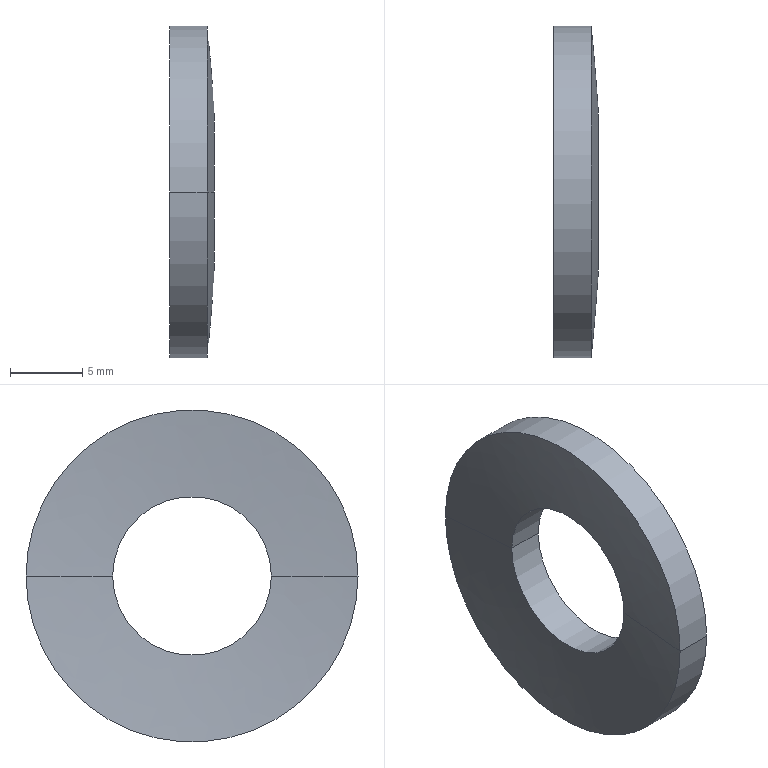Part | STEP file | M10_PAINE_LAATTA | 1 solid | 8 faces | box 3.1 x 23 x 23 mm | volume 834.027 mm3 | spline 4 | cylinder 4 | commonest cylinder face diameters 11 x2 23 x2
STEP:
#1=CARTESIAN_POINT('',(0.,0.,0.));
#2=DIRECTION('',(0.,0.,1.));
#3=DIRECTION('',(1.,0.,0.));
#4=AXIS2_PLACEMENT_3D('',#1,#2,#3);
#5=CARTESIAN_POINT('',(0.,11.5,0.));
#6=VERTEX_POINT('',#5);
#7=CARTESIAN_POINT('',(0.5,5.5,0.));
#8=VERTEX_POINT('',#7);
#9=CARTESIAN_POINT('',(-179.103,-6.446,0.));
#10=DIRECTION('',(0.,0.,-1.));
#11=DIRECTION('',(0.995,0.0997,0.));
#12=AXIS2_PLACEMENT_3D('',#9,#10,#11);
#13=CIRCLE('',#12,180.);
#14=CARTESIAN_POINT('',(-0.01205,11.597,-0.7296));
#15=CARTESIAN_POINT('',(0.1975,9.524,-0.5992));
#16=CARTESIAN_POINT('',(0.3708,7.448,-0.4686));
#17=CARTESIAN_POINT('',(0.508,5.369,-0.3378));
#18=CARTESIAN_POINT('',(-0.01205,12.046,6.407));
#19=CARTESIAN_POINT('',(0.1975,9.893,5.262));
#20=CARTESIAN_POINT('',(0.3708,7.736,4.115));
#21=CARTESIAN_POINT('',(0.508,5.577,2.966));
#22=CARTESIAN_POINT('',(-0.01205,7.151,11.62));
#23=CARTESIAN_POINT('',(0.1975,5.873,9.543));
#24=CARTESIAN_POINT('',(0.3708,4.593,7.463));
#25=CARTESIAN_POINT('',(0.508,3.311,5.38));
#26=CARTESIAN_POINT('',(-0.01205,0.,11.62));
#27=CARTESIAN_POINT('',(0.1975,0.,9.543));
#28=CARTESIAN_POINT('',(0.3708,0.,7.463));
#29=CARTESIAN_POINT('',(0.508,0.,5.38));
#30=CARTESIAN_POINT('',(-0.01205,-7.151,11.62));
#31=CARTESIAN_POINT('',(0.1975,-5.873,9.543));
#32=CARTESIAN_POINT('',(0.3708,-4.593,7.463));
#33=CARTESIAN_POINT('',(0.508,-3.311,5.38));
#34=CARTESIAN_POINT('',(-0.01205,-12.046,6.407));
#35=CARTESIAN_POINT('',(0.1975,-9.893,5.262));
#36=CARTESIAN_POINT('',(0.3708,-7.736,4.115));
#37=CARTESIAN_POINT('',(0.508,-5.577,2.966));
#38=CARTESIAN_POINT('',(-0.01205,-11.597,-0.7296));
#39=CARTESIAN_POINT('',(0.1975,-9.524,-0.5992));
#40=CARTESIAN_POINT('',(0.3708,-7.448,-0.4686));
#41=CARTESIAN_POINT('',(0.508,-5.369,-0.3378));
#42=(BOUNDED_SURFACE()B_SPLINE_SURFACE(3,3,((#14,#15,#16,#17),(#18,#19,#20,#21),(#22,#23,#24,#25),(#26,#27,#28,#29),(#30,#31,#32,#33),(#34,#35,#36,#37),(#38,#39,#40,#41)),.UNSPECIFIED.,.F.,.F.,.F.)B_SPLINE_SURFACE_WITH_KNOTS((4,3,4),(4,4),(0.,1.,2.),(0.,1.),.PIECEWISE_BEZIER_KNOTS.)GEOMETRIC_REPRESENTATION_ITEM()RATIONAL_B_SPLINE_SURFACE(((1.187,1.187,1.187,1.187),(0.9377,0.9376,0.9376,0.9377),(0.9377,0.9376,0.9376,0.9377),(1.187,1.187,1.187,1.187),(0.9377,0.9376,0.9376,0.9377),(0.9377,0.9376,0.9376,0.9377),(1.187,1.187,1.187,1.187)))REPRESENTATION_ITEM('')SURFACE());
#43=CARTESIAN_POINT('',(0.04253,0.01923));
#44=CARTESIAN_POINT('',(0.04253,0.9808));
#45=B_SPLINE_CURVE_WITH_KNOTS('',1,(#43,#44),.UNSPECIFIED.,.F.,.F.,(2,2),(0.,0.03345),.PIECEWISE_BEZIER_KNOTS.);
#46=(GEOMETRIC_REPRESENTATION_CONTEXT(2)PARAMETRIC_REPRESENTATION_CONTEXT()REPRESENTATION_CONTEXT('',''));
#47=DEFINITIONAL_REPRESENTATION('',(#45),#46);
#48=PCURVE('',#42,#47);
#49=CARTESIAN_POINT('',(-0.01205,-11.597,0.7296));
#50=CARTESIAN_POINT('',(0.1975,-9.524,0.5992));
#51=CARTESIAN_POINT('',(0.3708,-7.448,0.4686));
#52=CARTESIAN_POINT('',(0.508,-5.369,0.3378));
#53=CARTESIAN_POINT('',(-0.01205,-12.046,-6.407));
#54=CARTESIAN_POINT('',(0.1975,-9.893,-5.262));
#55=CARTESIAN_POINT('',(0.3708,-7.736,-4.115));
#56=CARTESIAN_POINT('',(0.508,-5.577,-2.966));
#57=CARTESIAN_POINT('',(-0.01205,-7.151,-11.62));
#58=CARTESIAN_POINT('',(0.1975,-5.873,-9.543));
#59=CARTESIAN_POINT('',(0.3708,-4.593,-7.463));
#60=CARTESIAN_POINT('',(0.508,-3.311,-5.38));
#61=CARTESIAN_POINT('',(-0.01205,0.,-11.62));
#62=CARTESIAN_POINT('',(0.1975,0.,-9.543));
#63=CARTESIAN_POINT('',(0.3708,0.,-7.463));
#64=CARTESIAN_POINT('',(0.508,0.,-5.38));
#65=CARTESIAN_POINT('',(-0.01205,7.151,-11.62));
#66=CARTESIAN_POINT('',(0.1975,5.873,-9.543));
#67=CARTESIAN_POINT('',(0.3708,4.593,-7.463));
#68=CARTESIAN_POINT('',(0.508,3.311,-5.38));
#69=CARTESIAN_POINT('',(-0.01205,12.046,-6.407));
#70=CARTESIAN_POINT('',(0.1975,9.893,-5.262));
#71=CARTESIAN_POINT('',(0.3708,7.736,-4.115));
#72=CARTESIAN_POINT('',(0.508,5.577,-2.966));
#73=CARTESIAN_POINT('',(-0.01205,11.597,0.7296));
#74=CARTESIAN_POINT('',(0.1975,9.524,0.5992));
#75=CARTESIAN_POINT('',(0.3708,7.448,0.4686));
#76=CARTESIAN_POINT('',(0.508,5.369,0.3378));
#77=(BOUNDED_SURFACE()B_SPLINE_SURFACE(3,3,((#49,#50,#51,#52),(#53,#54,#55,#56),(#57,#58,#59,#60),(#61,#62,#63,#64),(#65,#66,#67,#68),(#69,#70,#71,#72),(#73,#74,#75,#76)),.UNSPECIFIED.,.F.,.F.,.F.)B_SPLINE_SURFACE_WITH_KNOTS((4,3,4),(4,4),(0.,1.,2.),(0.,1.),.PIECEWISE_BEZIER_KNOTS.)GEOMETRIC_REPRESENTATION_ITEM()RATIONAL_B_SPLINE_SURFACE(((1.187,1.187,1.187,1.187),(0.9377,0.9376,0.9376,0.9377),(0.9377,0.9376,0.9376,0.9377),(1.187,1.187,1.187,1.187),(0.9377,0.9376,0.9376,0.9377),(0.9377,0.9376,0.9376,0.9377),(1.187,1.187,1.187,1.187)))REPRESENTATION_ITEM('')SURFACE());
#78=CARTESIAN_POINT('',(1.957,0.01923));
#79=CARTESIAN_POINT('',(1.957,0.9808));
#80=B_SPLINE_CURVE_WITH_KNOTS('',1,(#78,#79),.UNSPECIFIED.,.F.,.F.,(2,2),(0.,0.03345),.PIECEWISE_BEZIER_KNOTS.);
#81=(GEOMETRIC_REPRESENTATION_CONTEXT(2)PARAMETRIC_REPRESENTATION_CONTEXT()REPRESENTATION_CONTEXT('',''));
#82=DEFINITIONAL_REPRESENTATION('',(#80),#81);
#83=PCURVE('',#77,#82);
#84=SURFACE_CURVE('',#13,(#48,#83),.PCURVE_S1.);
#85=EDGE_CURVE('',#6,#8,#84,.T.);
#86=ORIENTED_EDGE('',*,*,#85,.F.);
#87=CARTESIAN_POINT('',(0.,-11.5,0.));
#88=VERTEX_POINT('',#87);
#89=CARTESIAN_POINT('',(0.,0.,0.));
#90=DIRECTION('',(1.,0.,0.));
#91=DIRECTION('',(0.,1.,0.));
#92=AXIS2_PLACEMENT_3D('',#89,#90,#91);
#93=CIRCLE('',#92,11.5);
#94=CARTESIAN_POINT('',(0.04253,0.01923));
#95=CARTESIAN_POINT('',(0.07433,0.01923));
#96=CARTESIAN_POINT('',(0.1362,0.01923));
#97=CARTESIAN_POINT('',(0.2248,0.01923));
#98=CARTESIAN_POINT('',(0.3106,0.01923));
#99=CARTESIAN_POINT('',(0.3943,0.01923));
#100=CARTESIAN_POINT('',(0.4769,0.01923));
#101=CARTESIAN_POINT('',(0.5593,0.01923));
#102=CARTESIAN_POINT('',(0.6424,0.01923));
#103=CARTESIAN_POINT('',(0.7268,0.01923));
#104=CARTESIAN_POINT('',(0.8138,0.01923));
#105=CARTESIAN_POINT('',(0.9038,0.01923));
#106=CARTESIAN_POINT('',(1.,0.01923));
#107=CARTESIAN_POINT('',(1.096,0.01923));
#108=CARTESIAN_POINT('',(1.186,0.01923));
#109=CARTESIAN_POINT('',(1.273,0.01923));
#110=CARTESIAN_POINT('',(1.358,0.01923));
#111=CARTESIAN_POINT('',(1.441,0.01923));
#112=CARTESIAN_POINT('',(1.523,0.01923));
#113=CARTESIAN_POINT('',(1.606,0.01923));
#114=CARTESIAN_POINT('',(1.689,0.01923));
#115=CARTESIAN_POINT('',(1.775,0.01923));
#116=CARTESIAN_POINT('',(1.864,0.01923));
#117=CARTESIAN_POINT('',(1.926,0.01923));
#118=CARTESIAN_POINT('',(1.957,0.01923));
#119=B_SPLINE_CURVE_WITH_KNOTS('',3,(#94,#95,#96,#97,#98,#99,#100,#101,#102,#103,#104,#105,#106,#107,#108,#109,#110,#111,#112,#113,#114,#115,#116,#117,#118),.UNSPECIFIED.,.F.,.F.,(4,1,1,1,1,1,1,1,1,1,1,1,1,1,1,1,1,1,1,1,1,1,4),(0.,0.1428,0.2856,0.4284,0.5712,0.714,0.8568,0.9996,1.142,1.285,1.428,1.571,1.714,1.856,1.999,2.142,2.285,2.428,2.57,2.713,2.856,2.999,3.142),.QUASI_UNIFORM_KNOTS.);
#120=(GEOMETRIC_REPRESENTATION_CONTEXT(2)PARAMETRIC_REPRESENTATION_CONTEXT()REPRESENTATION_CONTEXT('',''));
#121=DEFINITIONAL_REPRESENTATION('',(#119),#120);
#122=PCURVE('',#42,#121);
#123=CARTESIAN_POINT('',(-0.155,0.,0.));
#124=DIRECTION('',(1.,0.,0.));
#125=DIRECTION('',(0.,-1.,0.));
#126=AXIS2_PLACEMENT_3D('',#123,#124,#125);
#127=CYLINDRICAL_SURFACE('',#126,11.5);
#128=CARTESIAN_POINT('',(3.142,0.155));
#129=DIRECTION('',(1.,0.));
#130=VECTOR('',#129,1.);
#131=LINE('',#128,#130);
#132=(GEOMETRIC_REPRESENTATION_CONTEXT(2)PARAMETRIC_REPRESENTATION_CONTEXT()REPRESENTATION_CONTEXT('',''));
#133=DEFINITIONAL_REPRESENTATION('',(#131),#132);
#134=PCURVE('',#127,#133);
#135=SURFACE_CURVE('',#93,(#122,#134),.PCURVE_S1.);
#136=EDGE_CURVE('',#6,#88,#135,.T.);
#137=ORIENTED_EDGE('',*,*,#136,.T.);
#138=CARTESIAN_POINT('',(0.5,-5.5,0.));
#139=VERTEX_POINT('',#138);
#140=CARTESIAN_POINT('',(-179.103,6.446,0.));
#141=DIRECTION('',(0.,0.,1.));
#142=DIRECTION('',(0.995,-0.0997,0.));
#143=AXIS2_PLACEMENT_3D('',#140,#141,#142);
#144=CIRCLE('',#143,180.);
#145=CARTESIAN_POINT('',(1.957,0.01923));
#146=CARTESIAN_POINT('',(1.957,0.9808));
#147=B_SPLINE_CURVE_WITH_KNOTS('',1,(#145,#146),.UNSPECIFIED.,.F.,.F.,(2,2),(0.,0.03345),.PIECEWISE_BEZIER_KNOTS.);
#148=(GEOMETRIC_REPRESENTATION_CONTEXT(2)PARAMETRIC_REPRESENTATION_CONTEXT()REPRESENTATION_CONTEXT('',''));
#149=DEFINITIONAL_REPRESENTATION('',(#147),#148);
#150=PCURVE('',#42,#149);
#151=CARTESIAN_POINT('',(0.04253,0.01923));
#152=CARTESIAN_POINT('',(0.04253,0.9808));
#153=B_SPLINE_CURVE_WITH_KNOTS('',1,(#151,#152),.UNSPECIFIED.,.F.,.F.,(2,2),(0.,0.03345),.PIECEWISE_BEZIER_KNOTS.);
#154=(GEOMETRIC_REPRESENTATION_CONTEXT(2)PARAMETRIC_REPRESENTATION_CONTEXT()REPRESENTATION_CONTEXT('',''));
#155=DEFINITIONAL_REPRESENTATION('',(#153),#154);
#156=PCURVE('',#77,#155);
#157=SURFACE_CURVE('',#144,(#150,#156),.PCURVE_S1.);
#158=EDGE_CURVE('',#88,#139,#157,.T.);
#159=ORIENTED_EDGE('',*,*,#158,.T.);
#160=CARTESIAN_POINT('',(0.5,0.,0.));
#161=DIRECTION('',(1.,0.,0.));
#162=DIRECTION('',(0.,1.,0.));
#163=AXIS2_PLACEMENT_3D('',#160,#161,#162);
#164=CIRCLE('',#163,5.5);
#165=CARTESIAN_POINT('',(0.04253,0.9808));
#166=CARTESIAN_POINT('',(0.07433,0.9808));
#167=CARTESIAN_POINT('',(0.1362,0.9808));
#168=CARTESIAN_POINT('',(0.2248,0.9808));
#169=CARTESIAN_POINT('',(0.3106,0.9808));
#170=CARTESIAN_POINT('',(0.3943,0.9808));
#171=CARTESIAN_POINT('',(0.4769,0.9808));
#172=CARTESIAN_POINT('',(0.5593,0.9808));
#173=CARTESIAN_POINT('',(0.6424,0.9808));
#174=CARTESIAN_POINT('',(0.7268,0.9808));
#175=CARTESIAN_POINT('',(0.8138,0.9808));
#176=CARTESIAN_POINT('',(0.9038,0.9808));
#177=CARTESIAN_POINT('',(1.,0.9808));
#178=CARTESIAN_POINT('',(1.096,0.9808));
#179=CARTESIAN_POINT('',(1.186,0.9808));
#180=CARTESIAN_POINT('',(1.273,0.9808));
#181=CARTESIAN_POINT('',(1.358,0.9808));
#182=CARTESIAN_POINT('',(1.441,0.9808));
#183=CARTESIAN_POINT('',(1.523,0.9808));
#184=CARTESIAN_POINT('',(1.606,0.9808));
#185=CARTESIAN_POINT('',(1.689,0.9808));
#186=CARTESIAN_POINT('',(1.775,0.9808));
#187=CARTESIAN_POINT('',(1.864,0.9808));
#188=CARTESIAN_POINT('',(1.926,0.9808));
#189=CARTESIAN_POINT('',(1.957,0.9808));
#190=B_SPLINE_CURVE_WITH_KNOTS('',3,(#165,#166,#167,#168,#169,#170,#171,#172,#173,#174,#175,#176,#177,#178,#179,#180,#181,#182,#183,#184,#185,#186,#187,#188,#189),.UNSPECIFIED.,.F.,.F.,(4,1,1,1,1,1,1,1,1,1,1,1,1,1,1,1,1,1,1,1,1,1,4),(0.,0.1428,0.2856,0.4284,0.5712,0.714,0.8568,0.9996,1.142,1.285,1.428,1.571,1.714,1.856,1.999,2.142,2.285,2.428,2.57,2.713,2.856,2.999,3.142),.QUASI_UNIFORM_KNOTS.);
#191=(GEOMETRIC_REPRESENTATION_CONTEXT(2)PARAMETRIC_REPRESENTATION_CONTEXT()REPRESENTATION_CONTEXT('',''));
#192=DEFINITIONAL_REPRESENTATION('',(#190),#191);
#193=PCURVE('',#42,#192);
#194=CARTESIAN_POINT('',(-0.155,0.,0.));
#195=DIRECTION('',(1.,0.,0.));
#196=DIRECTION('',(0.,-1.,0.));
#197=AXIS2_PLACEMENT_3D('',#194,#195,#196);
#198=CYLINDRICAL_SURFACE('',#197,5.5);
#199=CARTESIAN_POINT('',(3.142,0.655));
#200=DIRECTION('',(1.,0.));
#201=VECTOR('',#200,1.);
#202=LINE('',#199,#201);
#203=(GEOMETRIC_REPRESENTATION_CONTEXT(2)PARAMETRIC_REPRESENTATION_CONTEXT()REPRESENTATION_CONTEXT('',''));
#204=DEFINITIONAL_REPRESENTATION('',(#202),#203);
#205=PCURVE('',#198,#204);
#206=SURFACE_CURVE('',#164,(#193,#205),.PCURVE_S1.);
#207=EDGE_CURVE('',#8,#139,#206,.T.);
#208=ORIENTED_EDGE('',*,*,#207,.F.);
#209=EDGE_LOOP('',(#86,#137,#159,#208));
#210=FACE_BOUND('',#209,.F.);
#211=ADVANCED_FACE('',(#210),#42,.F.);
#212=ORIENTED_EDGE('',*,*,#85,.T.);
#213=CARTESIAN_POINT('',(0.5,0.,0.));
#214=DIRECTION('',(-1.,0.,0.));
#215=DIRECTION('',(0.,1.,0.));
#216=AXIS2_PLACEMENT_3D('',#213,#214,#215);
#217=CIRCLE('',#216,5.5);
#218=CARTESIAN_POINT('',(1.957,0.9808));
#219=CARTESIAN_POINT('',(1.926,0.9808));
#220=CARTESIAN_POINT('',(1.864,0.9808));
#221=CARTESIAN_POINT('',(1.775,0.9808));
#222=CARTESIAN_POINT('',(1.689,0.9808));
#223=CARTESIAN_POINT('',(1.606,0.9808));
#224=CARTESIAN_POINT('',(1.523,0.9808));
#225=CARTESIAN_POINT('',(1.441,0.9808));
#226=CARTESIAN_POINT('',(1.358,0.9808));
#227=CARTESIAN_POINT('',(1.273,0.9808));
#228=CARTESIAN_POINT('',(1.186,0.9808));
#229=CARTESIAN_POINT('',(1.096,0.9808));
#230=CARTESIAN_POINT('',(1.,0.9808));
#231=CARTESIAN_POINT('',(0.9038,0.9808));
#232=CARTESIAN_POINT('',(0.8138,0.9808));
#233=CARTESIAN_POINT('',(0.7268,0.9808));
#234=CARTESIAN_POINT('',(0.6424,0.9808));
#235=CARTESIAN_POINT('',(0.5593,0.9808));
#236=CARTESIAN_POINT('',(0.4769,0.9808));
#237=CARTESIAN_POINT('',(0.3943,0.9808));
#238=CARTESIAN_POINT('',(0.3106,0.9808));
#239=CARTESIAN_POINT('',(0.2248,0.9808));
#240=CARTESIAN_POINT('',(0.1362,0.9808));
#241=CARTESIAN_POINT('',(0.07433,0.9808));
#242=CARTESIAN_POINT('',(0.04253,0.9808));
#243=B_SPLINE_CURVE_WITH_KNOTS('',3,(#218,#219,#220,#221,#222,#223,#224,#225,#226,#227,#228,#229,#230,#231,#232,#233,#234,#235,#236,#237,#238,#239,#240,#241,#242),.UNSPECIFIED.,.F.,.F.,(4,1,1,1,1,1,1,1,1,1,1,1,1,1,1,1,1,1,1,1,1,1,4),(0.,0.1428,0.2856,0.4284,0.5712,0.714,0.8568,0.9996,1.142,1.285,1.428,1.571,1.714,1.856,1.999,2.142,2.285,2.428,2.57,2.713,2.856,2.999,3.142),.QUASI_UNIFORM_KNOTS.);
#244=(GEOMETRIC_REPRESENTATION_CONTEXT(2)PARAMETRIC_REPRESENTATION_CONTEXT()REPRESENTATION_CONTEXT('',''));
#245=DEFINITIONAL_REPRESENTATION('',(#243),#244);
#246=PCURVE('',#77,#245);
#247=CARTESIAN_POINT('',(-0.155,0.,0.));
#248=DIRECTION('',(1.,0.,0.));
#249=DIRECTION('',(0.,-1.,0.));
#250=AXIS2_PLACEMENT_3D('',#247,#248,#249);
#251=CYLINDRICAL_SURFACE('',#250,5.5);
#252=CARTESIAN_POINT('',(3.142,0.655));
#253=DIRECTION('',(-1.,0.));
#254=VECTOR('',#253,1.);
#255=LINE('',#252,#254);
#256=(GEOMETRIC_REPRESENTATION_CONTEXT(2)PARAMETRIC_REPRESENTATION_CONTEXT()REPRESENTATION_CONTEXT('',''));
#257=DEFINITIONAL_REPRESENTATION('',(#255),#256);
#258=PCURVE('',#251,#257);
#259=SURFACE_CURVE('',#217,(#246,#258),.PCURVE_S1.);
#260=EDGE_CURVE('',#8,#139,#259,.T.);
#261=ORIENTED_EDGE('',*,*,#260,.T.);
#262=ORIENTED_EDGE('',*,*,#158,.F.);
#263=CARTESIAN_POINT('',(0.,0.,0.));
#264=DIRECTION('',(-1.,0.,0.));
#265=DIRECTION('',(0.,1.,0.));
#266=AXIS2_PLACEMENT_3D('',#263,#264,#265);
#267=CIRCLE('',#266,11.5);
#268=CARTESIAN_POINT('',(1.957,0.01923));
#269=CARTESIAN_POINT('',(1.926,0.01923));
#270=CARTESIAN_POINT('',(1.864,0.01923));
#271=CARTESIAN_POINT('',(1.775,0.01923));
#272=CARTESIAN_POINT('',(1.689,0.01923));
#273=CARTESIAN_POINT('',(1.606,0.01923));
#274=CARTESIAN_POINT('',(1.523,0.01923));
#275=CARTESIAN_POINT('',(1.441,0.01923));
#276=CARTESIAN_POINT('',(1.358,0.01923));
#277=CARTESIAN_POINT('',(1.273,0.01923));
#278=CARTESIAN_POINT('',(1.186,0.01923));
#279=CARTESIAN_POINT('',(1.096,0.01923));
#280=CARTESIAN_POINT('',(1.,0.01923));
#281=CARTESIAN_POINT('',(0.9038,0.01923));
#282=CARTESIAN_POINT('',(0.8138,0.01923));
#283=CARTESIAN_POINT('',(0.7268,0.01923));
#284=CARTESIAN_POINT('',(0.6424,0.01923));
#285=CARTESIAN_POINT('',(0.5593,0.01923));
#286=CARTESIAN_POINT('',(0.4769,0.01923));
#287=CARTESIAN_POINT('',(0.3943,0.01923));
#288=CARTESIAN_POINT('',(0.3106,0.01923));
#289=CARTESIAN_POINT('',(0.2248,0.01923));
#290=CARTESIAN_POINT('',(0.1362,0.01923));
#291=CARTESIAN_POINT('',(0.07433,0.01923));
#292=CARTESIAN_POINT('',(0.04253,0.01923));
#293=B_SPLINE_CURVE_WITH_KNOTS('',3,(#268,#269,#270,#271,#272,#273,#274,#275,#276,#277,#278,#279,#280,#281,#282,#283,#284,#285,#286,#287,#288,#289,#290,#291,#292),.UNSPECIFIED.,.F.,.F.,(4,1,1,1,1,1,1,1,1,1,1,1,1,1,1,1,1,1,1,1,1,1,4),(0.,0.1428,0.2856,0.4284,0.5712,0.714,0.8568,0.9996,1.142,1.285,1.428,1.571,1.714,1.856,1.999,2.142,2.285,2.428,2.57,2.713,2.856,2.999,3.142),.QUASI_UNIFORM_KNOTS.);
#294=(GEOMETRIC_REPRESENTATION_CONTEXT(2)PARAMETRIC_REPRESENTATION_CONTEXT()REPRESENTATION_CONTEXT('',''));
#295=DEFINITIONAL_REPRESENTATION('',(#293),#294);
#296=PCURVE('',#77,#295);
#297=CARTESIAN_POINT('',(-0.155,0.,0.));
#298=DIRECTION('',(1.,0.,0.));
#299=DIRECTION('',(0.,-1.,0.));
#300=AXIS2_PLACEMENT_3D('',#297,#298,#299);
#301=CYLINDRICAL_SURFACE('',#300,11.5);
#302=CARTESIAN_POINT('',(3.142,0.155));
#303=DIRECTION('',(-1.,0.));
#304=VECTOR('',#303,1.);
#305=LINE('',#302,#304);
#306=(GEOMETRIC_REPRESENTATION_CONTEXT(2)PARAMETRIC_REPRESENTATION_CONTEXT()REPRESENTATION_CONTEXT('',''));
#307=DEFINITIONAL_REPRESENTATION('',(#305),#306);
#308=PCURVE('',#301,#307);
#309=SURFACE_CURVE('',#267,(#296,#308),.PCURVE_S1.);
#310=EDGE_CURVE('',#6,#88,#309,.T.);
#311=ORIENTED_EDGE('',*,*,#310,.F.);
#312=EDGE_LOOP('',(#212,#261,#262,#311));
#313=FACE_BOUND('',#312,.F.);
#314=ADVANCED_FACE('',(#313),#77,.F.);
#315=CARTESIAN_POINT('',(3.1,5.5,0.));
#316=VERTEX_POINT('',#315);
#317=CARTESIAN_POINT('',(0.5,5.5,0.));
#318=DIRECTION('',(1.,0.,0.));
#319=VECTOR('',#318,1.);
#320=LINE('',#317,#319);
#321=CARTESIAN_POINT('',(3.142,0.655));
#322=DIRECTION('',(0.,1.));
#323=VECTOR('',#322,1.);
#324=LINE('',#321,#323);
#325=(GEOMETRIC_REPRESENTATION_CONTEXT(2)PARAMETRIC_REPRESENTATION_CONTEXT()REPRESENTATION_CONTEXT('',''));
#326=DEFINITIONAL_REPRESENTATION('',(#324),#325);
#327=PCURVE('',#251,#326);
#328=CARTESIAN_POINT('',(3.142,0.655));
#329=DIRECTION('',(0.,1.));
#330=VECTOR('',#329,1.);
#331=LINE('',#328,#330);
#332=(GEOMETRIC_REPRESENTATION_CONTEXT(2)PARAMETRIC_REPRESENTATION_CONTEXT()REPRESENTATION_CONTEXT('',''));
#333=DEFINITIONAL_REPRESENTATION('',(#331),#332);
#334=PCURVE('',#198,#333);
#335=SURFACE_CURVE('',#320,(#327,#334),.PCURVE_S1.);
#336=EDGE_CURVE('',#8,#316,#335,.T.);
#337=ORIENTED_EDGE('',*,*,#336,.T.);
#338=CARTESIAN_POINT('',(3.1,-5.5,0.));
#339=VERTEX_POINT('',#338);
#340=CARTESIAN_POINT('',(3.1,0.,0.));
#341=DIRECTION('',(-1.,0.,0.));
#342=DIRECTION('',(0.,1.,0.));
#343=AXIS2_PLACEMENT_3D('',#340,#341,#342);
#344=CIRCLE('',#343,5.5);
#345=CARTESIAN_POINT('',(3.142,3.255));
#346=DIRECTION('',(-1.,0.));
#347=VECTOR('',#346,1.);
#348=LINE('',#345,#347);
#349=(GEOMETRIC_REPRESENTATION_CONTEXT(2)PARAMETRIC_REPRESENTATION_CONTEXT()REPRESENTATION_CONTEXT('',''));
#350=DEFINITIONAL_REPRESENTATION('',(#348),#349);
#351=PCURVE('',#251,#350);
#352=CARTESIAN_POINT('',(2.588,-11.597,0.7296));
#353=CARTESIAN_POINT('',(2.797,-9.524,0.5992));
#354=CARTESIAN_POINT('',(2.971,-7.448,0.4686));
#355=CARTESIAN_POINT('',(3.108,-5.369,0.3378));
#356=CARTESIAN_POINT('',(2.588,-12.046,-6.407));
#357=CARTESIAN_POINT('',(2.797,-9.893,-5.262));
#358=CARTESIAN_POINT('',(2.971,-7.736,-4.115));
#359=CARTESIAN_POINT('',(3.108,-5.577,-2.966));
#360=CARTESIAN_POINT('',(2.588,-7.151,-11.62));
#361=CARTESIAN_POINT('',(2.797,-5.873,-9.543));
#362=CARTESIAN_POINT('',(2.971,-4.593,-7.463));
#363=CARTESIAN_POINT('',(3.108,-3.311,-5.38));
#364=CARTESIAN_POINT('',(2.588,0.,-11.62));
#365=CARTESIAN_POINT('',(2.797,0.,-9.543));
#366=CARTESIAN_POINT('',(2.971,0.,-7.463));
#367=CARTESIAN_POINT('',(3.108,0.,-5.38));
#368=CARTESIAN_POINT('',(2.588,7.151,-11.62));
#369=CARTESIAN_POINT('',(2.797,5.873,-9.543));
#370=CARTESIAN_POINT('',(2.971,4.593,-7.463));
#371=CARTESIAN_POINT('',(3.108,3.311,-5.38));
#372=CARTESIAN_POINT('',(2.588,12.046,-6.407));
#373=CARTESIAN_POINT('',(2.797,9.893,-5.262));
#374=CARTESIAN_POINT('',(2.971,7.736,-4.115));
#375=CARTESIAN_POINT('',(3.108,5.577,-2.966));
#376=CARTESIAN_POINT('',(2.588,11.597,0.7296));
#377=CARTESIAN_POINT('',(2.797,9.524,0.5992));
#378=CARTESIAN_POINT('',(2.971,7.448,0.4686));
#379=CARTESIAN_POINT('',(3.108,5.369,0.3378));
#380=(BOUNDED_SURFACE()B_SPLINE_SURFACE(3,3,((#352,#353,#354,#355),(#356,#357,#358,#359),(#360,#361,#362,#363),(#364,#365,#366,#367),(#368,#369,#370,#371),(#372,#373,#374,#375),(#376,#377,#378,#379)),.UNSPECIFIED.,.F.,.F.,.F.)B_SPLINE_SURFACE_WITH_KNOTS((4,3,4),(4,4),(0.,1.,2.),(0.,1.),.PIECEWISE_BEZIER_KNOTS.)GEOMETRIC_REPRESENTATION_ITEM()RATIONAL_B_SPLINE_SURFACE(((1.187,1.187,1.187,1.187),(0.9377,0.9376,0.9376,0.9377),(0.9377,0.9376,0.9376,0.9377),(1.187,1.187,1.187,1.187),(0.9377,0.9376,0.9376,0.9377),(0.9377,0.9376,0.9376,0.9377),(1.187,1.187,1.187,1.187)))REPRESENTATION_ITEM('')SURFACE());
#381=CARTESIAN_POINT('',(1.957,0.9808));
#382=CARTESIAN_POINT('',(1.926,0.9808));
#383=CARTESIAN_POINT('',(1.864,0.9808));
#384=CARTESIAN_POINT('',(1.775,0.9808));
#385=CARTESIAN_POINT('',(1.689,0.9808));
#386=CARTESIAN_POINT('',(1.606,0.9808));
#387=CARTESIAN_POINT('',(1.523,0.9808));
#388=CARTESIAN_POINT('',(1.441,0.9808));
#389=CARTESIAN_POINT('',(1.358,0.9808));
#390=CARTESIAN_POINT('',(1.273,0.9808));
#391=CARTESIAN_POINT('',(1.186,0.9808));
#392=CARTESIAN_POINT('',(1.096,0.9808));
#393=CARTESIAN_POINT('',(1.,0.9808));
#394=CARTESIAN_POINT('',(0.9038,0.9808));
#395=CARTESIAN_POINT('',(0.8138,0.9808));
#396=CARTESIAN_POINT('',(0.7268,0.9808));
#397=CARTESIAN_POINT('',(0.6424,0.9808));
#398=CARTESIAN_POINT('',(0.5593,0.9808));
#399=CARTESIAN_POINT('',(0.4769,0.9808));
#400=CARTESIAN_POINT('',(0.3943,0.9808));
#401=CARTESIAN_POINT('',(0.3106,0.9808));
#402=CARTESIAN_POINT('',(0.2248,0.9808));
#403=CARTESIAN_POINT('',(0.1362,0.9808));
#404=CARTESIAN_POINT('',(0.07433,0.9808));
#405=CARTESIAN_POINT('',(0.04253,0.9808));
#406=B_SPLINE_CURVE_WITH_KNOTS('',3,(#381,#382,#383,#384,#385,#386,#387,#388,#389,#390,#391,#392,#393,#394,#395,#396,#397,#398,#399,#400,#401,#402,#403,#404,#405),.UNSPECIFIED.,.F.,.F.,(4,1,1,1,1,1,1,1,1,1,1,1,1,1,1,1,1,1,1,1,1,1,4),(0.,0.1428,0.2856,0.4284,0.5712,0.714,0.8568,0.9996,1.142,1.285,1.428,1.571,1.714,1.856,1.999,2.142,2.285,2.428,2.57,2.713,2.856,2.999,3.142),.QUASI_UNIFORM_KNOTS.);
#407=(GEOMETRIC_REPRESENTATION_CONTEXT(2)PARAMETRIC_REPRESENTATION_CONTEXT()REPRESENTATION_CONTEXT('',''));
#408=DEFINITIONAL_REPRESENTATION('',(#406),#407);
#409=PCURVE('',#380,#408);
#410=SURFACE_CURVE('',#344,(#351,#409),.PCURVE_S1.);
#411=EDGE_CURVE('',#316,#339,#410,.T.);
#412=ORIENTED_EDGE('',*,*,#411,.T.);
#413=CARTESIAN_POINT('',(0.5,-5.5,0.));
#414=DIRECTION('',(1.,0.,0.));
#415=VECTOR('',#414,1.);
#416=LINE('',#413,#415);
#417=CARTESIAN_POINT('',(0.,0.655));
#418=DIRECTION('',(0.,1.));
#419=VECTOR('',#418,1.);
#420=LINE('',#417,#419);
#421=(GEOMETRIC_REPRESENTATION_CONTEXT(2)PARAMETRIC_REPRESENTATION_CONTEXT()REPRESENTATION_CONTEXT('',''));
#422=DEFINITIONAL_REPRESENTATION('',(#420),#421);
#423=PCURVE('',#251,#422);
#424=CARTESIAN_POINT('',(6.283,0.655));
#425=DIRECTION('',(0.,1.));
#426=VECTOR('',#425,1.);
#427=LINE('',#424,#426);
#428=(GEOMETRIC_REPRESENTATION_CONTEXT(2)PARAMETRIC_REPRESENTATION_CONTEXT()REPRESENTATION_CONTEXT('',''));
#429=DEFINITIONAL_REPRESENTATION('',(#427),#428);
#430=PCURVE('',#198,#429);
#431=SURFACE_CURVE('',#416,(#423,#430),.PCURVE_S1.);
#432=EDGE_CURVE('',#139,#339,#431,.T.);
#433=ORIENTED_EDGE('',*,*,#432,.F.);
#434=ORIENTED_EDGE('',*,*,#260,.F.);
#435=EDGE_LOOP('',(#337,#412,#433,#434));
#436=FACE_BOUND('',#435,.F.);
#437=ADVANCED_FACE('',(#436),#251,.F.);
#438=ORIENTED_EDGE('',*,*,#336,.F.);
#439=ORIENTED_EDGE('',*,*,#207,.T.);
#440=ORIENTED_EDGE('',*,*,#432,.T.);
#441=CARTESIAN_POINT('',(3.1,0.,0.));
#442=DIRECTION('',(1.,0.,0.));
#443=DIRECTION('',(0.,1.,0.));
#444=AXIS2_PLACEMENT_3D('',#441,#442,#443);
#445=CIRCLE('',#444,5.5);
#446=CARTESIAN_POINT('',(3.142,3.255));
#447=DIRECTION('',(1.,0.));
#448=VECTOR('',#447,1.);
#449=LINE('',#446,#448);
#450=(GEOMETRIC_REPRESENTATION_CONTEXT(2)PARAMETRIC_REPRESENTATION_CONTEXT()REPRESENTATION_CONTEXT('',''));
#451=DEFINITIONAL_REPRESENTATION('',(#449),#450);
#452=PCURVE('',#198,#451);
#453=CARTESIAN_POINT('',(2.588,11.597,-0.7296));
#454=CARTESIAN_POINT('',(2.797,9.524,-0.5992));
#455=CARTESIAN_POINT('',(2.971,7.448,-0.4686));
#456=CARTESIAN_POINT('',(3.108,5.369,-0.3378));
#457=CARTESIAN_POINT('',(2.588,12.046,6.407));
#458=CARTESIAN_POINT('',(2.797,9.893,5.262));
#459=CARTESIAN_POINT('',(2.971,7.736,4.115));
#460=CARTESIAN_POINT('',(3.108,5.577,2.966));
#461=CARTESIAN_POINT('',(2.588,7.151,11.62));
#462=CARTESIAN_POINT('',(2.797,5.873,9.543));
#463=CARTESIAN_POINT('',(2.971,4.593,7.463));
#464=CARTESIAN_POINT('',(3.108,3.311,5.38));
#465=CARTESIAN_POINT('',(2.588,0.,11.62));
#466=CARTESIAN_POINT('',(2.797,0.,9.543));
#467=CARTESIAN_POINT('',(2.971,0.,7.463));
#468=CARTESIAN_POINT('',(3.108,0.,5.38));
#469=CARTESIAN_POINT('',(2.588,-7.151,11.62));
#470=CARTESIAN_POINT('',(2.797,-5.873,9.543));
#471=CARTESIAN_POINT('',(2.971,-4.593,7.463));
#472=CARTESIAN_POINT('',(3.108,-3.311,5.38));
#473=CARTESIAN_POINT('',(2.588,-12.046,6.407));
#474=CARTESIAN_POINT('',(2.797,-9.893,5.262));
#475=CARTESIAN_POINT('',(2.971,-7.736,4.115));
#476=CARTESIAN_POINT('',(3.108,-5.577,2.966));
#477=CARTESIAN_POINT('',(2.588,-11.597,-0.7296));
#478=CARTESIAN_POINT('',(2.797,-9.524,-0.5992));
#479=CARTESIAN_POINT('',(2.971,-7.448,-0.4686));
#480=CARTESIAN_POINT('',(3.108,-5.369,-0.3378));
#481=(BOUNDED_SURFACE()B_SPLINE_SURFACE(3,3,((#453,#454,#455,#456),(#457,#458,#459,#460),(#461,#462,#463,#464),(#465,#466,#467,#468),(#469,#470,#471,#472),(#473,#474,#475,#476),(#477,#478,#479,#480)),.UNSPECIFIED.,.F.,.F.,.F.)B_SPLINE_SURFACE_WITH_KNOTS((4,3,4),(4,4),(0.,1.,2.),(0.,1.),.PIECEWISE_BEZIER_KNOTS.)GEOMETRIC_REPRESENTATION_ITEM()RATIONAL_B_SPLINE_SURFACE(((1.187,1.187,1.187,1.187),(0.9377,0.9376,0.9376,0.9377),(0.9377,0.9376,0.9376,0.9377),(1.187,1.187,1.187,1.187),(0.9377,0.9376,0.9376,0.9377),(0.9377,0.9376,0.9376,0.9377),(1.187,1.187,1.187,1.187)))REPRESENTATION_ITEM('')SURFACE());
#482=CARTESIAN_POINT('',(0.04253,0.9808));
#483=CARTESIAN_POINT('',(0.07433,0.9808));
#484=CARTESIAN_POINT('',(0.1362,0.9808));
#485=CARTESIAN_POINT('',(0.2248,0.9808));
#486=CARTESIAN_POINT('',(0.3106,0.9808));
#487=CARTESIAN_POINT('',(0.3943,0.9808));
#488=CARTESIAN_POINT('',(0.4769,0.9808));
#489=CARTESIAN_POINT('',(0.5593,0.9808));
#490=CARTESIAN_POINT('',(0.6424,0.9808));
#491=CARTESIAN_POINT('',(0.7268,0.9808));
#492=CARTESIAN_POINT('',(0.8138,0.9808));
#493=CARTESIAN_POINT('',(0.9038,0.9808));
#494=CARTESIAN_POINT('',(1.,0.9808));
#495=CARTESIAN_POINT('',(1.096,0.9808));
#496=CARTESIAN_POINT('',(1.186,0.9808));
#497=CARTESIAN_POINT('',(1.273,0.9808));
#498=CARTESIAN_POINT('',(1.358,0.9808));
#499=CARTESIAN_POINT('',(1.441,0.9808));
#500=CARTESIAN_POINT('',(1.523,0.9808));
#501=CARTESIAN_POINT('',(1.606,0.9808));
#502=CARTESIAN_POINT('',(1.689,0.9808));
#503=CARTESIAN_POINT('',(1.775,0.9808));
#504=CARTESIAN_POINT('',(1.864,0.9808));
#505=CARTESIAN_POINT('',(1.926,0.9808));
#506=CARTESIAN_POINT('',(1.957,0.9808));
#507=B_SPLINE_CURVE_WITH_KNOTS('',3,(#482,#483,#484,#485,#486,#487,#488,#489,#490,#491,#492,#493,#494,#495,#496,#497,#498,#499,#500,#501,#502,#503,#504,#505,#506),.UNSPECIFIED.,.F.,.F.,(4,1,1,1,1,1,1,1,1,1,1,1,1,1,1,1,1,1,1,1,1,1,4),(0.,0.1428,0.2856,0.4284,0.5712,0.714,0.8568,0.9996,1.142,1.285,1.428,1.571,1.714,1.856,1.999,2.142,2.285,2.428,2.57,2.713,2.856,2.999,3.142),.QUASI_UNIFORM_KNOTS.);
#508=(GEOMETRIC_REPRESENTATION_CONTEXT(2)PARAMETRIC_REPRESENTATION_CONTEXT()REPRESENTATION_CONTEXT('',''));
#509=DEFINITIONAL_REPRESENTATION('',(#507),#508);
#510=PCURVE('',#481,#509);
#511=SURFACE_CURVE('',#445,(#452,#510),.PCURVE_S1.);
#512=EDGE_CURVE('',#316,#339,#511,.T.);
#513=ORIENTED_EDGE('',*,*,#512,.F.);
#514=EDGE_LOOP('',(#438,#439,#440,#513));
#515=FACE_BOUND('',#514,.F.);
#516=ADVANCED_FACE('',(#515),#198,.F.);
#517=CARTESIAN_POINT('',(2.6,11.5,0.));
#518=VERTEX_POINT('',#517);
#519=CARTESIAN_POINT('',(2.6,-11.5,0.));
#520=VERTEX_POINT('',#519);
#521=CARTESIAN_POINT('',(2.6,0.,0.));
#522=DIRECTION('',(1.,0.,0.));
#523=DIRECTION('',(0.,1.,0.));
#524=AXIS2_PLACEMENT_3D('',#521,#522,#523);
#525=CIRCLE('',#524,11.5);
#526=CARTESIAN_POINT('',(0.04253,0.01923));
#527=CARTESIAN_POINT('',(0.07433,0.01923));
#528=CARTESIAN_POINT('',(0.1362,0.01923));
#529=CARTESIAN_POINT('',(0.2248,0.01923));
#530=CARTESIAN_POINT('',(0.3106,0.01923));
#531=CARTESIAN_POINT('',(0.3943,0.01923));
#532=CARTESIAN_POINT('',(0.4769,0.01923));
#533=CARTESIAN_POINT('',(0.5593,0.01923));
#534=CARTESIAN_POINT('',(0.6424,0.01923));
#535=CARTESIAN_POINT('',(0.7268,0.01923));
#536=CARTESIAN_POINT('',(0.8138,0.01923));
#537=CARTESIAN_POINT('',(0.9038,0.01923));
#538=CARTESIAN_POINT('',(1.,0.01923));
#539=CARTESIAN_POINT('',(1.096,0.01923));
#540=CARTESIAN_POINT('',(1.186,0.01923));
#541=CARTESIAN_POINT('',(1.273,0.01923));
#542=CARTESIAN_POINT('',(1.358,0.01923));
#543=CARTESIAN_POINT('',(1.441,0.01923));
#544=CARTESIAN_POINT('',(1.523,0.01923));
#545=CARTESIAN_POINT('',(1.606,0.01923));
#546=CARTESIAN_POINT('',(1.689,0.01923));
#547=CARTESIAN_POINT('',(1.775,0.01923));
#548=CARTESIAN_POINT('',(1.864,0.01923));
#549=CARTESIAN_POINT('',(1.926,0.01923));
#550=CARTESIAN_POINT('',(1.957,0.01923));
#551=B_SPLINE_CURVE_WITH_KNOTS('',3,(#526,#527,#528,#529,#530,#531,#532,#533,#534,#535,#536,#537,#538,#539,#540,#541,#542,#543,#544,#545,#546,#547,#548,#549,#550),.UNSPECIFIED.,.F.,.F.,(4,1,1,1,1,1,1,1,1,1,1,1,1,1,1,1,1,1,1,1,1,1,4),(0.,0.1428,0.2856,0.4284,0.5712,0.714,0.8568,0.9996,1.142,1.285,1.428,1.571,1.714,1.856,1.999,2.142,2.285,2.428,2.57,2.713,2.856,2.999,3.142),.QUASI_UNIFORM_KNOTS.);
#552=(GEOMETRIC_REPRESENTATION_CONTEXT(2)PARAMETRIC_REPRESENTATION_CONTEXT()REPRESENTATION_CONTEXT('',''));
#553=DEFINITIONAL_REPRESENTATION('',(#551),#552);
#554=PCURVE('',#481,#553);
#555=CARTESIAN_POINT('',(3.142,2.755));
#556=DIRECTION('',(1.,0.));
#557=VECTOR('',#556,1.);
#558=LINE('',#555,#557);
#559=(GEOMETRIC_REPRESENTATION_CONTEXT(2)PARAMETRIC_REPRESENTATION_CONTEXT()REPRESENTATION_CONTEXT('',''));
#560=DEFINITIONAL_REPRESENTATION('',(#558),#559);
#561=PCURVE('',#127,#560);
#562=SURFACE_CURVE('',#525,(#554,#561),.PCURVE_S1.);
#563=EDGE_CURVE('',#518,#520,#562,.T.);
#564=ORIENTED_EDGE('',*,*,#563,.T.);
#565=CARTESIAN_POINT('',(-176.503,6.446,0.));
#566=DIRECTION('',(0.,0.,-1.));
#567=DIRECTION('',(0.9978,-0.06637,0.));
#568=AXIS2_PLACEMENT_3D('',#565,#566,#567);
#569=CIRCLE('',#568,180.);
#570=CARTESIAN_POINT('',(1.957,0.9808));
#571=CARTESIAN_POINT('',(1.957,0.01923));
#572=B_SPLINE_CURVE_WITH_KNOTS('',1,(#570,#571),.UNSPECIFIED.,.F.,.F.,(2,2),(0.,0.03345),.PIECEWISE_BEZIER_KNOTS.);
#573=(GEOMETRIC_REPRESENTATION_CONTEXT(2)PARAMETRIC_REPRESENTATION_CONTEXT()REPRESENTATION_CONTEXT('',''));
#574=DEFINITIONAL_REPRESENTATION('',(#572),#573);
#575=PCURVE('',#481,#574);
#576=CARTESIAN_POINT('',(0.04253,0.9808));
#577=CARTESIAN_POINT('',(0.04253,0.01923));
#578=B_SPLINE_CURVE_WITH_KNOTS('',1,(#576,#577),.UNSPECIFIED.,.F.,.F.,(2,2),(0.,0.03345),.PIECEWISE_BEZIER_KNOTS.);
#579=(GEOMETRIC_REPRESENTATION_CONTEXT(2)PARAMETRIC_REPRESENTATION_CONTEXT()REPRESENTATION_CONTEXT('',''));
#580=DEFINITIONAL_REPRESENTATION('',(#578),#579);
#581=PCURVE('',#380,#580);
#582=SURFACE_CURVE('',#569,(#575,#581),.PCURVE_S1.);
#583=EDGE_CURVE('',#339,#520,#582,.T.);
#584=ORIENTED_EDGE('',*,*,#583,.F.);
#585=ORIENTED_EDGE('',*,*,#512,.F.);
#586=CARTESIAN_POINT('',(-176.503,-6.446,0.));
#587=DIRECTION('',(0.,0.,1.));
#588=DIRECTION('',(0.9978,0.06637,0.));
#589=AXIS2_PLACEMENT_3D('',#586,#587,#588);
#590=CIRCLE('',#589,180.);
#591=CARTESIAN_POINT('',(0.04253,0.9808));
#592=CARTESIAN_POINT('',(0.04253,0.01923));
#593=B_SPLINE_CURVE_WITH_KNOTS('',1,(#591,#592),.UNSPECIFIED.,.F.,.F.,(2,2),(0.,0.03345),.PIECEWISE_BEZIER_KNOTS.);
#594=(GEOMETRIC_REPRESENTATION_CONTEXT(2)PARAMETRIC_REPRESENTATION_CONTEXT()REPRESENTATION_CONTEXT('',''));
#595=DEFINITIONAL_REPRESENTATION('',(#593),#594);
#596=PCURVE('',#481,#595);
#597=CARTESIAN_POINT('',(1.957,0.9808));
#598=CARTESIAN_POINT('',(1.957,0.01923));
#599=B_SPLINE_CURVE_WITH_KNOTS('',1,(#597,#598),.UNSPECIFIED.,.F.,.F.,(2,2),(0.,0.03345),.PIECEWISE_BEZIER_KNOTS.);
#600=(GEOMETRIC_REPRESENTATION_CONTEXT(2)PARAMETRIC_REPRESENTATION_CONTEXT()REPRESENTATION_CONTEXT('',''));
#601=DEFINITIONAL_REPRESENTATION('',(#599),#600);
#602=PCURVE('',#380,#601);
#603=SURFACE_CURVE('',#590,(#596,#602),.PCURVE_S1.);
#604=EDGE_CURVE('',#316,#518,#603,.T.);
#605=ORIENTED_EDGE('',*,*,#604,.T.);
#606=EDGE_LOOP('',(#564,#584,#585,#605));
#607=FACE_BOUND('',#606,.T.);
#608=ADVANCED_FACE('',(#607),#481,.T.);
#609=ORIENTED_EDGE('',*,*,#411,.T.);
#610=ORIENTED_EDGE('',*,*,#583,.T.);
#611=CARTESIAN_POINT('',(2.6,0.,0.));
#612=DIRECTION('',(-1.,0.,0.));
#613=DIRECTION('',(0.,1.,0.));
#614=AXIS2_PLACEMENT_3D('',#611,#612,#613);
#615=CIRCLE('',#614,11.5);
#616=CARTESIAN_POINT('',(1.957,0.01923));
#617=CARTESIAN_POINT('',(1.926,0.01923));
#618=CARTESIAN_POINT('',(1.864,0.01923));
#619=CARTESIAN_POINT('',(1.775,0.01923));
#620=CARTESIAN_POINT('',(1.689,0.01923));
#621=CARTESIAN_POINT('',(1.606,0.01923));
#622=CARTESIAN_POINT('',(1.523,0.01923));
#623=CARTESIAN_POINT('',(1.441,0.01923));
#624=CARTESIAN_POINT('',(1.358,0.01923));
#625=CARTESIAN_POINT('',(1.273,0.01923));
#626=CARTESIAN_POINT('',(1.186,0.01923));
#627=CARTESIAN_POINT('',(1.096,0.01923));
#628=CARTESIAN_POINT('',(1.,0.01923));
#629=CARTESIAN_POINT('',(0.9038,0.01923));
#630=CARTESIAN_POINT('',(0.8138,0.01923));
#631=CARTESIAN_POINT('',(0.7268,0.01923));
#632=CARTESIAN_POINT('',(0.6424,0.01923));
#633=CARTESIAN_POINT('',(0.5593,0.01923));
#634=CARTESIAN_POINT('',(0.4769,0.01923));
#635=CARTESIAN_POINT('',(0.3943,0.01923));
#636=CARTESIAN_POINT('',(0.3106,0.01923));
#637=CARTESIAN_POINT('',(0.2248,0.01923));
#638=CARTESIAN_POINT('',(0.1362,0.01923));
#639=CARTESIAN_POINT('',(0.07433,0.01923));
#640=CARTESIAN_POINT('',(0.04253,0.01923));
#641=B_SPLINE_CURVE_WITH_KNOTS('',3,(#616,#617,#618,#619,#620,#621,#622,#623,#624,#625,#626,#627,#628,#629,#630,#631,#632,#633,#634,#635,#636,#637,#638,#639,#640),.UNSPECIFIED.,.F.,.F.,(4,1,1,1,1,1,1,1,1,1,1,1,1,1,1,1,1,1,1,1,1,1,4),(0.,0.1428,0.2856,0.4284,0.5712,0.714,0.8568,0.9996,1.142,1.285,1.428,1.571,1.714,1.856,1.999,2.142,2.285,2.428,2.57,2.713,2.856,2.999,3.142),.QUASI_UNIFORM_KNOTS.);
#642=(GEOMETRIC_REPRESENTATION_CONTEXT(2)PARAMETRIC_REPRESENTATION_CONTEXT()REPRESENTATION_CONTEXT('',''));
#643=DEFINITIONAL_REPRESENTATION('',(#641),#642);
#644=PCURVE('',#380,#643);
#645=CARTESIAN_POINT('',(3.142,2.755));
#646=DIRECTION('',(-1.,0.));
#647=VECTOR('',#646,1.);
#648=LINE('',#645,#647);
#649=(GEOMETRIC_REPRESENTATION_CONTEXT(2)PARAMETRIC_REPRESENTATION_CONTEXT()REPRESENTATION_CONTEXT('',''));
#650=DEFINITIONAL_REPRESENTATION('',(#648),#649);
#651=PCURVE('',#301,#650);
#652=SURFACE_CURVE('',#615,(#644,#651),.PCURVE_S1.);
#653=EDGE_CURVE('',#518,#520,#652,.T.);
#654=ORIENTED_EDGE('',*,*,#653,.F.);
#655=ORIENTED_EDGE('',*,*,#604,.F.);
#656=EDGE_LOOP('',(#609,#610,#654,#655));
#657=FACE_BOUND('',#656,.T.);
#658=ADVANCED_FACE('',(#657),#380,.T.);
#659=ORIENTED_EDGE('',*,*,#653,.T.);
#660=CARTESIAN_POINT('',(2.6,-11.5,0.));
#661=DIRECTION('',(-1.,0.,0.));
#662=VECTOR('',#661,1.);
#663=LINE('',#660,#662);
#664=CARTESIAN_POINT('',(0.,2.755));
#665=DIRECTION('',(0.,-1.));
#666=VECTOR('',#665,1.);
#667=LINE('',#664,#666);
#668=(GEOMETRIC_REPRESENTATION_CONTEXT(2)PARAMETRIC_REPRESENTATION_CONTEXT()REPRESENTATION_CONTEXT('',''));
#669=DEFINITIONAL_REPRESENTATION('',(#667),#668);
#670=PCURVE('',#301,#669);
#671=CARTESIAN_POINT('',(6.283,2.755));
#672=DIRECTION('',(0.,-1.));
#673=VECTOR('',#672,1.);
#674=LINE('',#671,#673);
#675=(GEOMETRIC_REPRESENTATION_CONTEXT(2)PARAMETRIC_REPRESENTATION_CONTEXT()REPRESENTATION_CONTEXT('',''));
#676=DEFINITIONAL_REPRESENTATION('',(#674),#675);
#677=PCURVE('',#127,#676);
#678=SURFACE_CURVE('',#663,(#670,#677),.PCURVE_S1.);
#679=EDGE_CURVE('',#520,#88,#678,.T.);
#680=ORIENTED_EDGE('',*,*,#679,.T.);
#681=ORIENTED_EDGE('',*,*,#310,.F.);
#682=CARTESIAN_POINT('',(2.6,11.5,0.));
#683=DIRECTION('',(-1.,0.,0.));
#684=VECTOR('',#683,1.);
#685=LINE('',#682,#684);
#686=CARTESIAN_POINT('',(3.142,2.755));
#687=DIRECTION('',(0.,-1.));
#688=VECTOR('',#687,1.);
#689=LINE('',#686,#688);
#690=(GEOMETRIC_REPRESENTATION_CONTEXT(2)PARAMETRIC_REPRESENTATION_CONTEXT()REPRESENTATION_CONTEXT('',''));
#691=DEFINITIONAL_REPRESENTATION('',(#689),#690);
#692=PCURVE('',#301,#691);
#693=CARTESIAN_POINT('',(3.142,2.755));
#694=DIRECTION('',(0.,-1.));
#695=VECTOR('',#694,1.);
#696=LINE('',#693,#695);
#697=(GEOMETRIC_REPRESENTATION_CONTEXT(2)PARAMETRIC_REPRESENTATION_CONTEXT()REPRESENTATION_CONTEXT('',''));
#698=DEFINITIONAL_REPRESENTATION('',(#696),#697);
#699=PCURVE('',#127,#698);
#700=SURFACE_CURVE('',#685,(#692,#699),.PCURVE_S1.);
#701=EDGE_CURVE('',#518,#6,#700,.T.);
#702=ORIENTED_EDGE('',*,*,#701,.F.);
#703=EDGE_LOOP('',(#659,#680,#681,#702));
#704=FACE_BOUND('',#703,.T.);
#705=ADVANCED_FACE('',(#704),#301,.T.);
#706=ORIENTED_EDGE('',*,*,#136,.T.);
#707=ORIENTED_EDGE('',*,*,#679,.F.);
#708=ORIENTED_EDGE('',*,*,#563,.F.);
#709=ORIENTED_EDGE('',*,*,#701,.T.);
#710=EDGE_LOOP('',(#706,#707,#708,#709));
#711=FACE_BOUND('',#710,.T.);
#712=ADVANCED_FACE('',(#711),#127,.T.);
#713=CLOSED_SHELL('',(#211,#314,#437,#516,#608,#658,#705,#712));
#714=MANIFOLD_SOLID_BREP('',#713);
#715=(LENGTH_UNIT()NAMED_UNIT(*)SI_UNIT(.MILLI.,.METRE.));
#716=UNCERTAINTY_MEASURE_WITH_UNIT(LENGTH_MEASURE(0.00002),#715,'','');
#717=(NAMED_UNIT(*)PLANE_ANGLE_UNIT()SI_UNIT($,.RADIAN.));
#718=(NAMED_UNIT(*)SI_UNIT($,.STERADIAN.)SOLID_ANGLE_UNIT());
#719=(GEOMETRIC_REPRESENTATION_CONTEXT(3)GLOBAL_UNCERTAINTY_ASSIGNED_CONTEXT((#716))GLOBAL_UNIT_ASSIGNED_CONTEXT((#715,#717,#718))REPRESENTATION_CONTEXT('',''));
#720=ADVANCED_BREP_SHAPE_REPRESENTATION('',(#4,#714),#719);